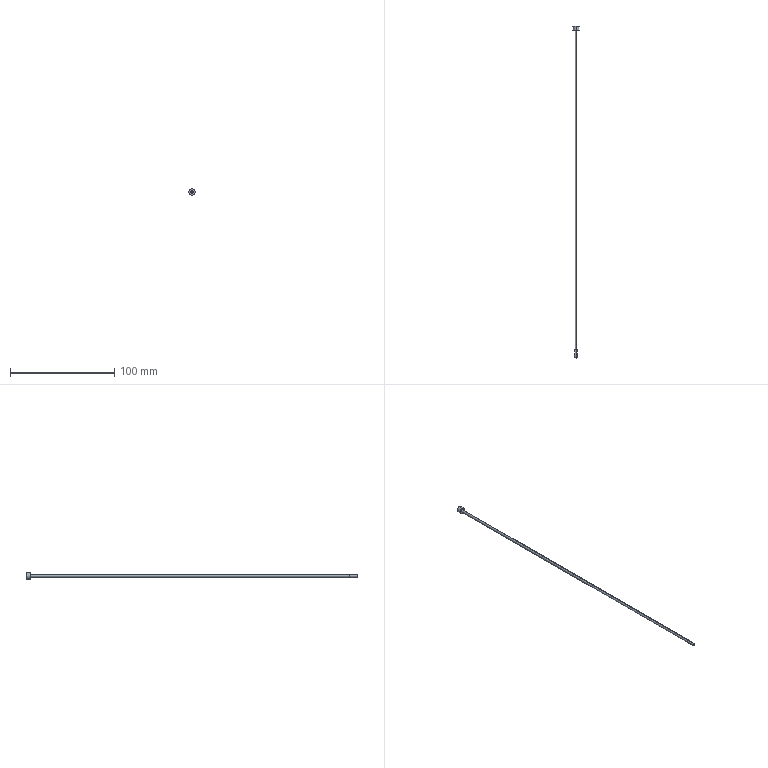Part | STEP file | 1 solid | 9 faces | box 6 x 317.863 x 6 mm | volume 1651 mm3 | cylinder 4 | plane 3 | cone 2 | commonest cylinder face diameters 2.5 x2 6 x2
STEP:
#1=CARTESIAN_POINT('',(0.,0.,0.));
#2=DIRECTION('',(0.,0.,1.));
#3=DIRECTION('',(1.,0.,0.));
#4=AXIS2_PLACEMENT_3D('',#1,#2,#3);
#5=CARTESIAN_POINT('',(-129.143,345.5,185.94));
#6=VERTEX_POINT('',#5);
#7=CARTESIAN_POINT('',(-129.143,345.5,191.94));
#8=VERTEX_POINT('',#7);
#9=CARTESIAN_POINT('',(-129.143,345.5,188.94));
#10=DIRECTION('',(0.,-1.,0.));
#11=DIRECTION('',(0.,0.,-1.));
#12=AXIS2_PLACEMENT_3D('',#9,#10,#11);
#13=CIRCLE('',#12,3.);
#14=CARTESIAN_POINT('',(-129.143,345.5,188.94));
#15=DIRECTION('',(0.,-1.,0.));
#16=DIRECTION('',(0.,0.,-1.));
#17=AXIS2_PLACEMENT_3D('',#14,#15,#16);
#18=CYLINDRICAL_SURFACE('',#17,3.);
#19=CARTESIAN_POINT('',(0.,0.));
#20=DIRECTION('',(1.,0.));
#21=VECTOR('',#20,1.);
#22=LINE('',#19,#21);
#23=(GEOMETRIC_REPRESENTATION_CONTEXT(2)PARAMETRIC_REPRESENTATION_CONTEXT()REPRESENTATION_CONTEXT('',''));
#24=DEFINITIONAL_REPRESENTATION('',(#22),#23);
#25=PCURVE('',#18,#24);
#26=CARTESIAN_POINT('',(-72.862,345.5,110.196));
#27=DIRECTION('',(0.,-1.,0.));
#28=DIRECTION('',(0.,0.,-1.));
#29=AXIS2_PLACEMENT_3D('',#26,#27,#28);
#30=PLANE('',#29);
#31=CARTESIAN_POINT('',(-78.744,-56.28));
#32=DIRECTION('',(1.,0.));
#33=AXIS2_PLACEMENT_2D('',#31,#32);
#34=CIRCLE('',#33,3.);
#35=(GEOMETRIC_REPRESENTATION_CONTEXT(2)PARAMETRIC_REPRESENTATION_CONTEXT()REPRESENTATION_CONTEXT('',''));
#36=DEFINITIONAL_REPRESENTATION('',(#34),#35);
#37=PCURVE('',#30,#36);
#38=SURFACE_CURVE('',#13,(#25,#37),.PCURVE_S1.);
#39=EDGE_CURVE('',#6,#8,#38,.T.);
#40=ORIENTED_EDGE('',*,*,#39,.T.);
#41=CARTESIAN_POINT('',(-129.143,341.5,191.94));
#42=VERTEX_POINT('',#41);
#43=CARTESIAN_POINT('',(-129.143,345.5,191.94));
#44=DIRECTION('',(0.,-1.,0.));
#45=VECTOR('',#44,1.);
#46=LINE('',#43,#45);
#47=CARTESIAN_POINT('',(3.142,0.));
#48=DIRECTION('',(0.,1.));
#49=VECTOR('',#48,1.);
#50=LINE('',#47,#49);
#51=(GEOMETRIC_REPRESENTATION_CONTEXT(2)PARAMETRIC_REPRESENTATION_CONTEXT()REPRESENTATION_CONTEXT('',''));
#52=DEFINITIONAL_REPRESENTATION('',(#50),#51);
#53=PCURVE('',#18,#52);
#54=CARTESIAN_POINT('',(-129.143,345.5,188.94));
#55=DIRECTION('',(0.,-1.,0.));
#56=DIRECTION('',(0.,0.,-1.));
#57=AXIS2_PLACEMENT_3D('',#54,#55,#56);
#58=CYLINDRICAL_SURFACE('',#57,3.);
#59=CARTESIAN_POINT('',(3.142,0.));
#60=DIRECTION('',(0.,1.));
#61=VECTOR('',#60,1.);
#62=LINE('',#59,#61);
#63=(GEOMETRIC_REPRESENTATION_CONTEXT(2)PARAMETRIC_REPRESENTATION_CONTEXT()REPRESENTATION_CONTEXT('',''));
#64=DEFINITIONAL_REPRESENTATION('',(#62),#63);
#65=PCURVE('',#58,#64);
#66=SURFACE_CURVE('',#46,(#53,#65),.PCURVE_S1.);
#67=EDGE_CURVE('',#8,#42,#66,.T.);
#68=ORIENTED_EDGE('',*,*,#67,.T.);
#69=CARTESIAN_POINT('',(-129.143,341.5,185.94));
#70=VERTEX_POINT('',#69);
#71=CARTESIAN_POINT('',(-129.143,341.5,188.94));
#72=DIRECTION('',(0.,1.,0.));
#73=DIRECTION('',(0.,0.,1.));
#74=AXIS2_PLACEMENT_3D('',#71,#72,#73);
#75=CIRCLE('',#74,3.);
#76=CARTESIAN_POINT('',(3.142,4.));
#77=DIRECTION('',(-1.,0.));
#78=VECTOR('',#77,1.);
#79=LINE('',#76,#78);
#80=(GEOMETRIC_REPRESENTATION_CONTEXT(2)PARAMETRIC_REPRESENTATION_CONTEXT()REPRESENTATION_CONTEXT('',''));
#81=DEFINITIONAL_REPRESENTATION('',(#79),#80);
#82=PCURVE('',#18,#81);
#83=CARTESIAN_POINT('',(-129.143,341.5,188.94));
#84=DIRECTION('',(0.,-1.,0.));
#85=DIRECTION('',(0.,0.,-1.));
#86=AXIS2_PLACEMENT_3D('',#83,#84,#85);
#87=PLANE('',#86);
#88=CARTESIAN_POINT('',(-3.,0.));
#89=CARTESIAN_POINT('',(-3.,5.196));
#90=CARTESIAN_POINT('',(1.5,2.598));
#91=CARTESIAN_POINT('',(6.,0.));
#92=CARTESIAN_POINT('',(1.5,-2.598));
#93=CARTESIAN_POINT('',(-3.,-5.196));
#94=CARTESIAN_POINT('',(-3.,0.));
#95=(BOUNDED_CURVE()B_SPLINE_CURVE(2,(#88,#89,#90,#91,#92,#93,#94),.UNSPECIFIED.,.T.,.F.)B_SPLINE_CURVE_WITH_KNOTS((1,2,2,2,2,1),(-2.094,0.,2.094,4.189,6.283,8.378),.UNSPECIFIED.)CURVE()GEOMETRIC_REPRESENTATION_ITEM()RATIONAL_B_SPLINE_CURVE((1.,0.5,1.,0.5,1.,0.5,1.))REPRESENTATION_ITEM(''));
#96=(GEOMETRIC_REPRESENTATION_CONTEXT(2)PARAMETRIC_REPRESENTATION_CONTEXT()REPRESENTATION_CONTEXT('',''));
#97=DEFINITIONAL_REPRESENTATION('',(#95),#96);
#98=PCURVE('',#87,#97);
#99=SURFACE_CURVE('',#75,(#82,#98),.PCURVE_S1.);
#100=EDGE_CURVE('',#42,#70,#99,.T.);
#101=ORIENTED_EDGE('',*,*,#100,.T.);
#102=CARTESIAN_POINT('',(-129.143,345.5,185.94));
#103=DIRECTION('',(0.,-1.,0.));
#104=VECTOR('',#103,1.);
#105=LINE('',#102,#104);
#106=CARTESIAN_POINT('',(0.,0.));
#107=DIRECTION('',(0.,1.));
#108=VECTOR('',#107,1.);
#109=LINE('',#106,#108);
#110=(GEOMETRIC_REPRESENTATION_CONTEXT(2)PARAMETRIC_REPRESENTATION_CONTEXT()REPRESENTATION_CONTEXT('',''));
#111=DEFINITIONAL_REPRESENTATION('',(#109),#110);
#112=PCURVE('',#18,#111);
#113=CARTESIAN_POINT('',(6.283,0.));
#114=DIRECTION('',(0.,1.));
#115=VECTOR('',#114,1.);
#116=LINE('',#113,#115);
#117=(GEOMETRIC_REPRESENTATION_CONTEXT(2)PARAMETRIC_REPRESENTATION_CONTEXT()REPRESENTATION_CONTEXT('',''));
#118=DEFINITIONAL_REPRESENTATION('',(#116),#117);
#119=PCURVE('',#58,#118);
#120=SURFACE_CURVE('',#105,(#112,#119),.PCURVE_S1.);
#121=EDGE_CURVE('',#6,#70,#120,.T.);
#122=ORIENTED_EDGE('',*,*,#121,.F.);
#123=EDGE_LOOP('',(#40,#68,#101,#122));
#124=FACE_BOUND('',#123,.T.);
#125=ADVANCED_FACE('',(#124),#18,.T.);
#126=CARTESIAN_POINT('',(-129.143,27.637,190.117));
#127=VERTEX_POINT('',#126);
#128=CARTESIAN_POINT('',(-129.143,27.637,187.763));
#129=VERTEX_POINT('',#128);
#130=CARTESIAN_POINT('',(-129.143,27.637,188.94));
#131=DIRECTION('',(0.,1.,0.));
#132=DIRECTION('',(0.,0.,1.));
#133=AXIS2_PLACEMENT_3D('',#130,#131,#132);
#134=CIRCLE('',#133,1.177);
#135=CARTESIAN_POINT('',(-129.143,36.682,188.94));
#136=DIRECTION('',(0.,1.,0.));
#137=DIRECTION('',(0.,0.,1.));
#138=AXIS2_PLACEMENT_3D('',#135,#136,#137);
#139=CONICAL_SURFACE('',#138,1.256,0.008727);
#140=CARTESIAN_POINT('',(0.,-9.045));
#141=DIRECTION('',(1.,0.));
#142=VECTOR('',#141,1.);
#143=LINE('',#140,#142);
#144=(GEOMETRIC_REPRESENTATION_CONTEXT(2)PARAMETRIC_REPRESENTATION_CONTEXT()REPRESENTATION_CONTEXT('',''));
#145=DEFINITIONAL_REPRESENTATION('',(#143),#144);
#146=PCURVE('',#139,#145);
#147=CARTESIAN_POINT('',(-129.143,27.637,188.94));
#148=DIRECTION('',(0.,-1.,0.));
#149=DIRECTION('',(0.,0.,-1.));
#150=AXIS2_PLACEMENT_3D('',#147,#148,#149);
#151=PLANE('',#150);
#152=CARTESIAN_POINT('',(-1.177,0.));
#153=CARTESIAN_POINT('',(-1.177,2.039));
#154=CARTESIAN_POINT('',(0.5887,1.02));
#155=CARTESIAN_POINT('',(2.355,0.));
#156=CARTESIAN_POINT('',(0.5887,-1.02));
#157=CARTESIAN_POINT('',(-1.177,-2.039));
#158=CARTESIAN_POINT('',(-1.177,0.));
#159=(BOUNDED_CURVE()B_SPLINE_CURVE(2,(#152,#153,#154,#155,#156,#157,#158),.UNSPECIFIED.,.T.,.F.)B_SPLINE_CURVE_WITH_KNOTS((1,2,2,2,2,1),(-2.094,0.,2.094,4.189,6.283,8.378),.UNSPECIFIED.)CURVE()GEOMETRIC_REPRESENTATION_ITEM()RATIONAL_B_SPLINE_CURVE((1.,0.5,1.,0.5,1.,0.5,1.))REPRESENTATION_ITEM(''));
#160=(GEOMETRIC_REPRESENTATION_CONTEXT(2)PARAMETRIC_REPRESENTATION_CONTEXT()REPRESENTATION_CONTEXT('',''));
#161=DEFINITIONAL_REPRESENTATION('',(#159),#160);
#162=PCURVE('',#151,#161);
#163=SURFACE_CURVE('',#134,(#146,#162),.PCURVE_S1.);
#164=EDGE_CURVE('',#127,#129,#163,.T.);
#165=ORIENTED_EDGE('',*,*,#164,.T.);
#166=CARTESIAN_POINT('',(-129.143,35.966,187.69));
#167=VERTEX_POINT('',#166);
#168=CARTESIAN_POINT('',(-129.143,36.682,187.684));
#169=DIRECTION('',(0.,1.,-0.008727));
#170=VECTOR('',#169,1.);
#171=LINE('',#168,#170);
#172=CARTESIAN_POINT('',(3.142,0.));
#173=DIRECTION('',(0.,1.));
#174=VECTOR('',#173,1.);
#175=LINE('',#172,#174);
#176=(GEOMETRIC_REPRESENTATION_CONTEXT(2)PARAMETRIC_REPRESENTATION_CONTEXT()REPRESENTATION_CONTEXT('',''));
#177=DEFINITIONAL_REPRESENTATION('',(#175),#176);
#178=PCURVE('',#139,#177);
#179=CARTESIAN_POINT('',(-129.143,36.682,188.94));
#180=DIRECTION('',(0.,1.,0.));
#181=DIRECTION('',(0.,0.,1.));
#182=AXIS2_PLACEMENT_3D('',#179,#180,#181);
#183=CONICAL_SURFACE('',#182,1.256,0.008727);
#184=CARTESIAN_POINT('',(3.142,0.));
#185=DIRECTION('',(0.,1.));
#186=VECTOR('',#185,1.);
#187=LINE('',#184,#186);
#188=(GEOMETRIC_REPRESENTATION_CONTEXT(2)PARAMETRIC_REPRESENTATION_CONTEXT()REPRESENTATION_CONTEXT('',''));
#189=DEFINITIONAL_REPRESENTATION('',(#187),#188);
#190=PCURVE('',#183,#189);
#191=SURFACE_CURVE('',#171,(#178,#190),.PCURVE_S1.);
#192=EDGE_CURVE('',#129,#167,#191,.T.);
#193=ORIENTED_EDGE('',*,*,#192,.T.);
#194=CARTESIAN_POINT('',(-129.143,35.966,190.19));
#195=VERTEX_POINT('',#194);
#196=CARTESIAN_POINT('',(-129.143,35.966,188.94));
#197=DIRECTION('',(0.,1.,0.));
#198=DIRECTION('',(0.,0.,1.));
#199=AXIS2_PLACEMENT_3D('',#196,#197,#198);
#200=CIRCLE('',#199,1.25);
#201=CARTESIAN_POINT('',(0.,-0.7162));
#202=DIRECTION('',(1.,0.));
#203=VECTOR('',#202,1.);
#204=LINE('',#201,#203);
#205=(GEOMETRIC_REPRESENTATION_CONTEXT(2)PARAMETRIC_REPRESENTATION_CONTEXT()REPRESENTATION_CONTEXT('',''));
#206=DEFINITIONAL_REPRESENTATION('',(#204),#205);
#207=PCURVE('',#139,#206);
#208=CARTESIAN_POINT('',(-129.143,27.637,188.94));
#209=DIRECTION('',(0.,1.,0.));
#210=DIRECTION('',(0.,0.,1.));
#211=AXIS2_PLACEMENT_3D('',#208,#209,#210);
#212=CYLINDRICAL_SURFACE('',#211,1.25);
#213=CARTESIAN_POINT('',(0.,8.329));
#214=DIRECTION('',(1.,0.));
#215=VECTOR('',#214,1.);
#216=LINE('',#213,#215);
#217=(GEOMETRIC_REPRESENTATION_CONTEXT(2)PARAMETRIC_REPRESENTATION_CONTEXT()REPRESENTATION_CONTEXT('',''));
#218=DEFINITIONAL_REPRESENTATION('',(#216),#217);
#219=PCURVE('',#212,#218);
#220=SURFACE_CURVE('',#200,(#207,#219),.PCURVE_S1.);
#221=EDGE_CURVE('',#195,#167,#220,.T.);
#222=ORIENTED_EDGE('',*,*,#221,.F.);
#223=CARTESIAN_POINT('',(-129.143,36.682,190.196));
#224=DIRECTION('',(0.,1.,0.008727));
#225=VECTOR('',#224,1.);
#226=LINE('',#223,#225);
#227=CARTESIAN_POINT('',(0.,0.));
#228=DIRECTION('',(0.,1.));
#229=VECTOR('',#228,1.);
#230=LINE('',#227,#229);
#231=(GEOMETRIC_REPRESENTATION_CONTEXT(2)PARAMETRIC_REPRESENTATION_CONTEXT()REPRESENTATION_CONTEXT('',''));
#232=DEFINITIONAL_REPRESENTATION('',(#230),#231);
#233=PCURVE('',#139,#232);
#234=CARTESIAN_POINT('',(6.283,0.));
#235=DIRECTION('',(0.,1.));
#236=VECTOR('',#235,1.);
#237=LINE('',#234,#236);
#238=(GEOMETRIC_REPRESENTATION_CONTEXT(2)PARAMETRIC_REPRESENTATION_CONTEXT()REPRESENTATION_CONTEXT('',''));
#239=DEFINITIONAL_REPRESENTATION('',(#237),#238);
#240=PCURVE('',#183,#239);
#241=SURFACE_CURVE('',#226,(#233,#240),.PCURVE_S1.);
#242=EDGE_CURVE('',#127,#195,#241,.T.);
#243=ORIENTED_EDGE('',*,*,#242,.F.);
#244=EDGE_LOOP('',(#165,#193,#222,#243));
#245=FACE_BOUND('',#244,.T.);
#246=ADVANCED_FACE('',(#245),#139,.T.);
#247=ORIENTED_EDGE('',*,*,#221,.T.);
#248=CARTESIAN_POINT('',(-129.143,341.5,187.69));
#249=VERTEX_POINT('',#248);
#250=CARTESIAN_POINT('',(-129.143,27.637,187.69));
#251=DIRECTION('',(0.,1.,0.));
#252=VECTOR('',#251,1.);
#253=LINE('',#250,#252);
#254=CARTESIAN_POINT('',(3.142,0.));
#255=DIRECTION('',(0.,1.));
#256=VECTOR('',#255,1.);
#257=LINE('',#254,#256);
#258=(GEOMETRIC_REPRESENTATION_CONTEXT(2)PARAMETRIC_REPRESENTATION_CONTEXT()REPRESENTATION_CONTEXT('',''));
#259=DEFINITIONAL_REPRESENTATION('',(#257),#258);
#260=PCURVE('',#212,#259);
#261=CARTESIAN_POINT('',(-129.143,27.637,188.94));
#262=DIRECTION('',(0.,1.,0.));
#263=DIRECTION('',(0.,0.,1.));
#264=AXIS2_PLACEMENT_3D('',#261,#262,#263);
#265=CYLINDRICAL_SURFACE('',#264,1.25);
#266=CARTESIAN_POINT('',(3.142,0.));
#267=DIRECTION('',(0.,1.));
#268=VECTOR('',#267,1.);
#269=LINE('',#266,#268);
#270=(GEOMETRIC_REPRESENTATION_CONTEXT(2)PARAMETRIC_REPRESENTATION_CONTEXT()REPRESENTATION_CONTEXT('',''));
#271=DEFINITIONAL_REPRESENTATION('',(#269),#270);
#272=PCURVE('',#265,#271);
#273=SURFACE_CURVE('',#253,(#260,#272),.PCURVE_S1.);
#274=EDGE_CURVE('',#167,#249,#273,.T.);
#275=ORIENTED_EDGE('',*,*,#274,.T.);
#276=CARTESIAN_POINT('',(-129.143,341.5,190.19));
#277=VERTEX_POINT('',#276);
#278=CARTESIAN_POINT('',(-129.143,341.5,188.94));
#279=DIRECTION('',(0.,1.,0.));
#280=DIRECTION('',(0.,0.,-1.));
#281=AXIS2_PLACEMENT_3D('',#278,#279,#280);
#282=CIRCLE('',#281,1.25);
#283=CARTESIAN_POINT('',(-3.142,313.863));
#284=DIRECTION('',(1.,0.));
#285=VECTOR('',#284,1.);
#286=LINE('',#283,#285);
#287=(GEOMETRIC_REPRESENTATION_CONTEXT(2)PARAMETRIC_REPRESENTATION_CONTEXT()REPRESENTATION_CONTEXT('',''));
#288=DEFINITIONAL_REPRESENTATION('',(#286),#287);
#289=PCURVE('',#212,#288);
#290=CARTESIAN_POINT('',(1.25,0.));
#291=CARTESIAN_POINT('',(1.25,-2.165));
#292=CARTESIAN_POINT('',(-0.625,-1.083));
#293=CARTESIAN_POINT('',(-2.5,0.));
#294=CARTESIAN_POINT('',(-0.625,1.083));
#295=CARTESIAN_POINT('',(1.25,2.165));
#296=CARTESIAN_POINT('',(1.25,0.));
#297=(BOUNDED_CURVE()B_SPLINE_CURVE(2,(#290,#291,#292,#293,#294,#295,#296),.UNSPECIFIED.,.T.,.F.)B_SPLINE_CURVE_WITH_KNOTS((1,2,2,2,2,1),(-2.094,0.,2.094,4.189,6.283,8.378),.UNSPECIFIED.)CURVE()GEOMETRIC_REPRESENTATION_ITEM()RATIONAL_B_SPLINE_CURVE((1.,0.5,1.,0.5,1.,0.5,1.))REPRESENTATION_ITEM(''));
#298=(GEOMETRIC_REPRESENTATION_CONTEXT(2)PARAMETRIC_REPRESENTATION_CONTEXT()REPRESENTATION_CONTEXT('',''));
#299=DEFINITIONAL_REPRESENTATION('',(#297),#298);
#300=PCURVE('',#87,#299);
#301=SURFACE_CURVE('',#282,(#289,#300),.PCURVE_S1.);
#302=EDGE_CURVE('',#277,#249,#301,.T.);
#303=ORIENTED_EDGE('',*,*,#302,.F.);
#304=CARTESIAN_POINT('',(-129.143,27.637,190.19));
#305=DIRECTION('',(0.,1.,0.));
#306=VECTOR('',#305,1.);
#307=LINE('',#304,#306);
#308=CARTESIAN_POINT('',(0.,0.));
#309=DIRECTION('',(0.,1.));
#310=VECTOR('',#309,1.);
#311=LINE('',#308,#310);
#312=(GEOMETRIC_REPRESENTATION_CONTEXT(2)PARAMETRIC_REPRESENTATION_CONTEXT()REPRESENTATION_CONTEXT('',''));
#313=DEFINITIONAL_REPRESENTATION('',(#311),#312);
#314=PCURVE('',#212,#313);
#315=CARTESIAN_POINT('',(6.283,0.));
#316=DIRECTION('',(0.,1.));
#317=VECTOR('',#316,1.);
#318=LINE('',#315,#317);
#319=(GEOMETRIC_REPRESENTATION_CONTEXT(2)PARAMETRIC_REPRESENTATION_CONTEXT()REPRESENTATION_CONTEXT('',''));
#320=DEFINITIONAL_REPRESENTATION('',(#318),#319);
#321=PCURVE('',#265,#320);
#322=SURFACE_CURVE('',#307,(#314,#321),.PCURVE_S1.);
#323=EDGE_CURVE('',#195,#277,#322,.T.);
#324=ORIENTED_EDGE('',*,*,#323,.F.);
#325=EDGE_LOOP('',(#247,#275,#303,#324));
#326=FACE_BOUND('',#325,.T.);
#327=ADVANCED_FACE('',(#326),#212,.T.);
#328=ORIENTED_EDGE('',*,*,#274,.F.);
#329=CARTESIAN_POINT('',(-129.143,35.966,188.94));
#330=DIRECTION('',(0.,1.,0.));
#331=DIRECTION('',(0.,0.,1.));
#332=AXIS2_PLACEMENT_3D('',#329,#330,#331);
#333=CIRCLE('',#332,1.25);
#334=CARTESIAN_POINT('',(0.,8.329));
#335=DIRECTION('',(1.,0.));
#336=VECTOR('',#335,1.);
#337=LINE('',#334,#336);
#338=(GEOMETRIC_REPRESENTATION_CONTEXT(2)PARAMETRIC_REPRESENTATION_CONTEXT()REPRESENTATION_CONTEXT('',''));
#339=DEFINITIONAL_REPRESENTATION('',(#337),#338);
#340=PCURVE('',#265,#339);
#341=CARTESIAN_POINT('',(0.,-0.7162));
#342=DIRECTION('',(1.,0.));
#343=VECTOR('',#342,1.);
#344=LINE('',#341,#343);
#345=(GEOMETRIC_REPRESENTATION_CONTEXT(2)PARAMETRIC_REPRESENTATION_CONTEXT()REPRESENTATION_CONTEXT('',''));
#346=DEFINITIONAL_REPRESENTATION('',(#344),#345);
#347=PCURVE('',#183,#346);
#348=SURFACE_CURVE('',#333,(#340,#347),.PCURVE_S1.);
#349=EDGE_CURVE('',#167,#195,#348,.T.);
#350=ORIENTED_EDGE('',*,*,#349,.T.);
#351=ORIENTED_EDGE('',*,*,#323,.T.);
#352=CARTESIAN_POINT('',(-129.143,341.5,188.94));
#353=DIRECTION('',(0.,1.,0.));
#354=DIRECTION('',(0.,0.,-1.));
#355=AXIS2_PLACEMENT_3D('',#352,#353,#354);
#356=CIRCLE('',#355,1.25);
#357=CARTESIAN_POINT('',(3.142,313.863));
#358=DIRECTION('',(1.,0.));
#359=VECTOR('',#358,1.);
#360=LINE('',#357,#359);
#361=(GEOMETRIC_REPRESENTATION_CONTEXT(2)PARAMETRIC_REPRESENTATION_CONTEXT()REPRESENTATION_CONTEXT('',''));
#362=DEFINITIONAL_REPRESENTATION('',(#360),#361);
#363=PCURVE('',#265,#362);
#364=CARTESIAN_POINT('',(1.25,0.));
#365=CARTESIAN_POINT('',(1.25,-2.165));
#366=CARTESIAN_POINT('',(-0.625,-1.083));
#367=CARTESIAN_POINT('',(-2.5,0.));
#368=CARTESIAN_POINT('',(-0.625,1.083));
#369=CARTESIAN_POINT('',(1.25,2.165));
#370=CARTESIAN_POINT('',(1.25,0.));
#371=(BOUNDED_CURVE()B_SPLINE_CURVE(2,(#364,#365,#366,#367,#368,#369,#370),.UNSPECIFIED.,.T.,.F.)B_SPLINE_CURVE_WITH_KNOTS((1,2,2,2,2,1),(-2.094,0.,2.094,4.189,6.283,8.378),.UNSPECIFIED.)CURVE()GEOMETRIC_REPRESENTATION_ITEM()RATIONAL_B_SPLINE_CURVE((1.,0.5,1.,0.5,1.,0.5,1.))REPRESENTATION_ITEM(''));
#372=(GEOMETRIC_REPRESENTATION_CONTEXT(2)PARAMETRIC_REPRESENTATION_CONTEXT()REPRESENTATION_CONTEXT('',''));
#373=DEFINITIONAL_REPRESENTATION('',(#371),#372);
#374=PCURVE('',#87,#373);
#375=SURFACE_CURVE('',#356,(#363,#374),.PCURVE_S1.);
#376=EDGE_CURVE('',#249,#277,#375,.T.);
#377=ORIENTED_EDGE('',*,*,#376,.F.);
#378=EDGE_LOOP('',(#328,#350,#351,#377));
#379=FACE_BOUND('',#378,.T.);
#380=ADVANCED_FACE('',(#379),#265,.T.);
#381=ORIENTED_EDGE('',*,*,#192,.F.);
#382=CARTESIAN_POINT('',(-129.143,27.637,188.94));
#383=DIRECTION('',(0.,1.,0.));
#384=DIRECTION('',(0.,0.,1.));
#385=AXIS2_PLACEMENT_3D('',#382,#383,#384);
#386=CIRCLE('',#385,1.177);
#387=CARTESIAN_POINT('',(0.,-9.045));
#388=DIRECTION('',(1.,0.));
#389=VECTOR('',#388,1.);
#390=LINE('',#387,#389);
#391=(GEOMETRIC_REPRESENTATION_CONTEXT(2)PARAMETRIC_REPRESENTATION_CONTEXT()REPRESENTATION_CONTEXT('',''));
#392=DEFINITIONAL_REPRESENTATION('',(#390),#391);
#393=PCURVE('',#183,#392);
#394=CARTESIAN_POINT('',(-1.177,0.));
#395=CARTESIAN_POINT('',(-1.177,2.039));
#396=CARTESIAN_POINT('',(0.5887,1.02));
#397=CARTESIAN_POINT('',(2.355,0.));
#398=CARTESIAN_POINT('',(0.5887,-1.02));
#399=CARTESIAN_POINT('',(-1.177,-2.039));
#400=CARTESIAN_POINT('',(-1.177,0.));
#401=(BOUNDED_CURVE()B_SPLINE_CURVE(2,(#394,#395,#396,#397,#398,#399,#400),.UNSPECIFIED.,.T.,.F.)B_SPLINE_CURVE_WITH_KNOTS((1,2,2,2,2,1),(-2.094,0.,2.094,4.189,6.283,8.378),.UNSPECIFIED.)CURVE()GEOMETRIC_REPRESENTATION_ITEM()RATIONAL_B_SPLINE_CURVE((1.,0.5,1.,0.5,1.,0.5,1.))REPRESENTATION_ITEM(''));
#402=(GEOMETRIC_REPRESENTATION_CONTEXT(2)PARAMETRIC_REPRESENTATION_CONTEXT()REPRESENTATION_CONTEXT('',''));
#403=DEFINITIONAL_REPRESENTATION('',(#401),#402);
#404=PCURVE('',#151,#403);
#405=SURFACE_CURVE('',#386,(#393,#404),.PCURVE_S1.);
#406=EDGE_CURVE('',#129,#127,#405,.T.);
#407=ORIENTED_EDGE('',*,*,#406,.T.);
#408=ORIENTED_EDGE('',*,*,#242,.T.);
#409=ORIENTED_EDGE('',*,*,#349,.F.);
#410=EDGE_LOOP('',(#381,#407,#408,#409));
#411=FACE_BOUND('',#410,.T.);
#412=ADVANCED_FACE('',(#411),#183,.T.);
#413=ORIENTED_EDGE('',*,*,#164,.F.);
#414=ORIENTED_EDGE('',*,*,#406,.F.);
#415=EDGE_LOOP('',(#413,#414));
#416=FACE_BOUND('',#415,.T.);
#417=ADVANCED_FACE('',(#416),#151,.T.);
#418=ORIENTED_EDGE('',*,*,#302,.T.);
#419=ORIENTED_EDGE('',*,*,#376,.T.);
#420=EDGE_LOOP('',(#418,#419));
#421=FACE_BOUND('',#420,.T.);
#422=CARTESIAN_POINT('',(-129.143,341.5,188.94));
#423=DIRECTION('',(0.,1.,0.));
#424=DIRECTION('',(0.,0.,1.));
#425=AXIS2_PLACEMENT_3D('',#422,#423,#424);
#426=CIRCLE('',#425,3.);
#427=CARTESIAN_POINT('',(-3.,0.));
#428=CARTESIAN_POINT('',(-3.,5.196));
#429=CARTESIAN_POINT('',(1.5,2.598));
#430=CARTESIAN_POINT('',(6.,0.));
#431=CARTESIAN_POINT('',(1.5,-2.598));
#432=CARTESIAN_POINT('',(-3.,-5.196));
#433=CARTESIAN_POINT('',(-3.,0.));
#434=(BOUNDED_CURVE()B_SPLINE_CURVE(2,(#427,#428,#429,#430,#431,#432,#433),.UNSPECIFIED.,.T.,.F.)B_SPLINE_CURVE_WITH_KNOTS((1,2,2,2,2,1),(-2.094,0.,2.094,4.189,6.283,8.378),.UNSPECIFIED.)CURVE()GEOMETRIC_REPRESENTATION_ITEM()RATIONAL_B_SPLINE_CURVE((1.,0.5,1.,0.5,1.,0.5,1.))REPRESENTATION_ITEM(''));
#435=(GEOMETRIC_REPRESENTATION_CONTEXT(2)PARAMETRIC_REPRESENTATION_CONTEXT()REPRESENTATION_CONTEXT('',''));
#436=DEFINITIONAL_REPRESENTATION('',(#434),#435);
#437=PCURVE('',#87,#436);
#438=CARTESIAN_POINT('',(9.425,4.));
#439=DIRECTION('',(-1.,0.));
#440=VECTOR('',#439,1.);
#441=LINE('',#438,#440);
#442=(GEOMETRIC_REPRESENTATION_CONTEXT(2)PARAMETRIC_REPRESENTATION_CONTEXT()REPRESENTATION_CONTEXT('',''));
#443=DEFINITIONAL_REPRESENTATION('',(#441),#442);
#444=PCURVE('',#58,#443);
#445=SURFACE_CURVE('',#426,(#437,#444),.PCURVE_S1.);
#446=EDGE_CURVE('',#70,#42,#445,.T.);
#447=ORIENTED_EDGE('',*,*,#446,.F.);
#448=ORIENTED_EDGE('',*,*,#100,.F.);
#449=EDGE_LOOP('',(#447,#448));
#450=FACE_BOUND('',#449,.T.);
#451=ADVANCED_FACE('',(#421,#450),#87,.T.);
#452=ORIENTED_EDGE('',*,*,#67,.F.);
#453=CARTESIAN_POINT('',(-129.143,345.5,188.94));
#454=DIRECTION('',(0.,-1.,0.));
#455=DIRECTION('',(0.,0.,-1.));
#456=AXIS2_PLACEMENT_3D('',#453,#454,#455);
#457=CIRCLE('',#456,3.);
#458=CARTESIAN_POINT('',(0.,0.));
#459=DIRECTION('',(1.,0.));
#460=VECTOR('',#459,1.);
#461=LINE('',#458,#460);
#462=(GEOMETRIC_REPRESENTATION_CONTEXT(2)PARAMETRIC_REPRESENTATION_CONTEXT()REPRESENTATION_CONTEXT('',''));
#463=DEFINITIONAL_REPRESENTATION('',(#461),#462);
#464=PCURVE('',#58,#463);
#465=CARTESIAN_POINT('',(-78.744,-56.28));
#466=DIRECTION('',(1.,0.));
#467=AXIS2_PLACEMENT_2D('',#465,#466);
#468=CIRCLE('',#467,3.);
#469=(GEOMETRIC_REPRESENTATION_CONTEXT(2)PARAMETRIC_REPRESENTATION_CONTEXT()REPRESENTATION_CONTEXT('',''));
#470=DEFINITIONAL_REPRESENTATION('',(#468),#469);
#471=PCURVE('',#30,#470);
#472=SURFACE_CURVE('',#457,(#464,#471),.PCURVE_S1.);
#473=EDGE_CURVE('',#8,#6,#472,.T.);
#474=ORIENTED_EDGE('',*,*,#473,.T.);
#475=ORIENTED_EDGE('',*,*,#121,.T.);
#476=ORIENTED_EDGE('',*,*,#446,.T.);
#477=EDGE_LOOP('',(#452,#474,#475,#476));
#478=FACE_BOUND('',#477,.T.);
#479=ADVANCED_FACE('',(#478),#58,.T.);
#480=ORIENTED_EDGE('',*,*,#39,.F.);
#481=ORIENTED_EDGE('',*,*,#473,.F.);
#482=EDGE_LOOP('',(#480,#481));
#483=FACE_BOUND('',#482,.T.);
#484=ADVANCED_FACE('',(#483),#30,.F.);
#485=CLOSED_SHELL('',(#125,#246,#327,#380,#412,#417,#451,#479,#484));
#486=MANIFOLD_SOLID_BREP('',#485);
#487=(LENGTH_UNIT()NAMED_UNIT(*)SI_UNIT(.MILLI.,.METRE.));
#488=UNCERTAINTY_MEASURE_WITH_UNIT(LENGTH_MEASURE(0.0000001),#487,'','');
#489=(NAMED_UNIT(*)PLANE_ANGLE_UNIT()SI_UNIT($,.RADIAN.));
#490=(NAMED_UNIT(*)SI_UNIT($,.STERADIAN.)SOLID_ANGLE_UNIT());
#491=(GEOMETRIC_REPRESENTATION_CONTEXT(3)GLOBAL_UNCERTAINTY_ASSIGNED_CONTEXT((#488))GLOBAL_UNIT_ASSIGNED_CONTEXT((#487,#489,#490))REPRESENTATION_CONTEXT('',''));
#492=ADVANCED_BREP_SHAPE_REPRESENTATION('',(#4,#486),#491);